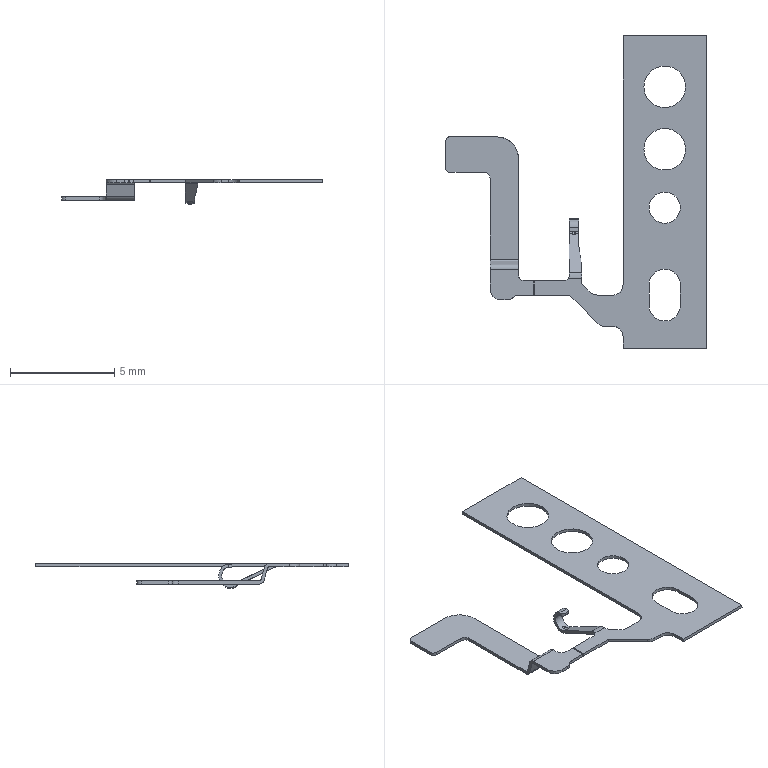Part | STEP file | p9-frame-05 | 1 solid | 85 faces | box 12.521 x 15 x 1.199 mm | volume 10.626 mm3 | plane 41 | cylinder 33 | spline 11 | commonest cylinder face diameters 0.602 x6 1.5 x5 2 x4 0.401 x3 0.201 x2 0.301 x2